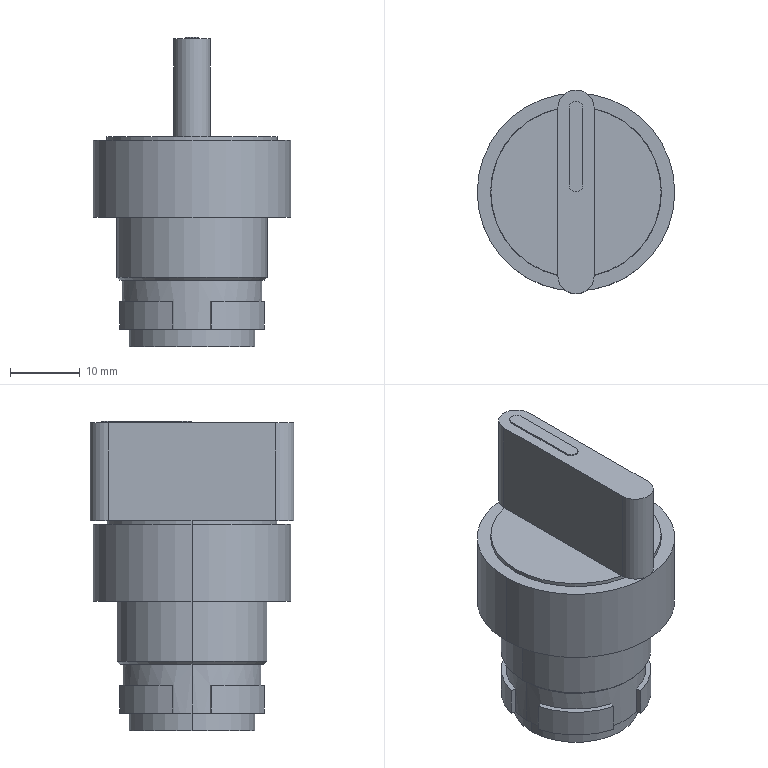Part | STEP file | 001. Schneider two-position switch XB2-BD21C | 1 solid | 61 faces | box 28.3 x 29.2 x 44.3 mm | volume 13844 mm3 | plane 33 | cylinder 26 | cone 2 | commonest cylinder face diameters 21.5 x6 1.985 x2 2 x2 5.2 x2 11 x2 18 x2